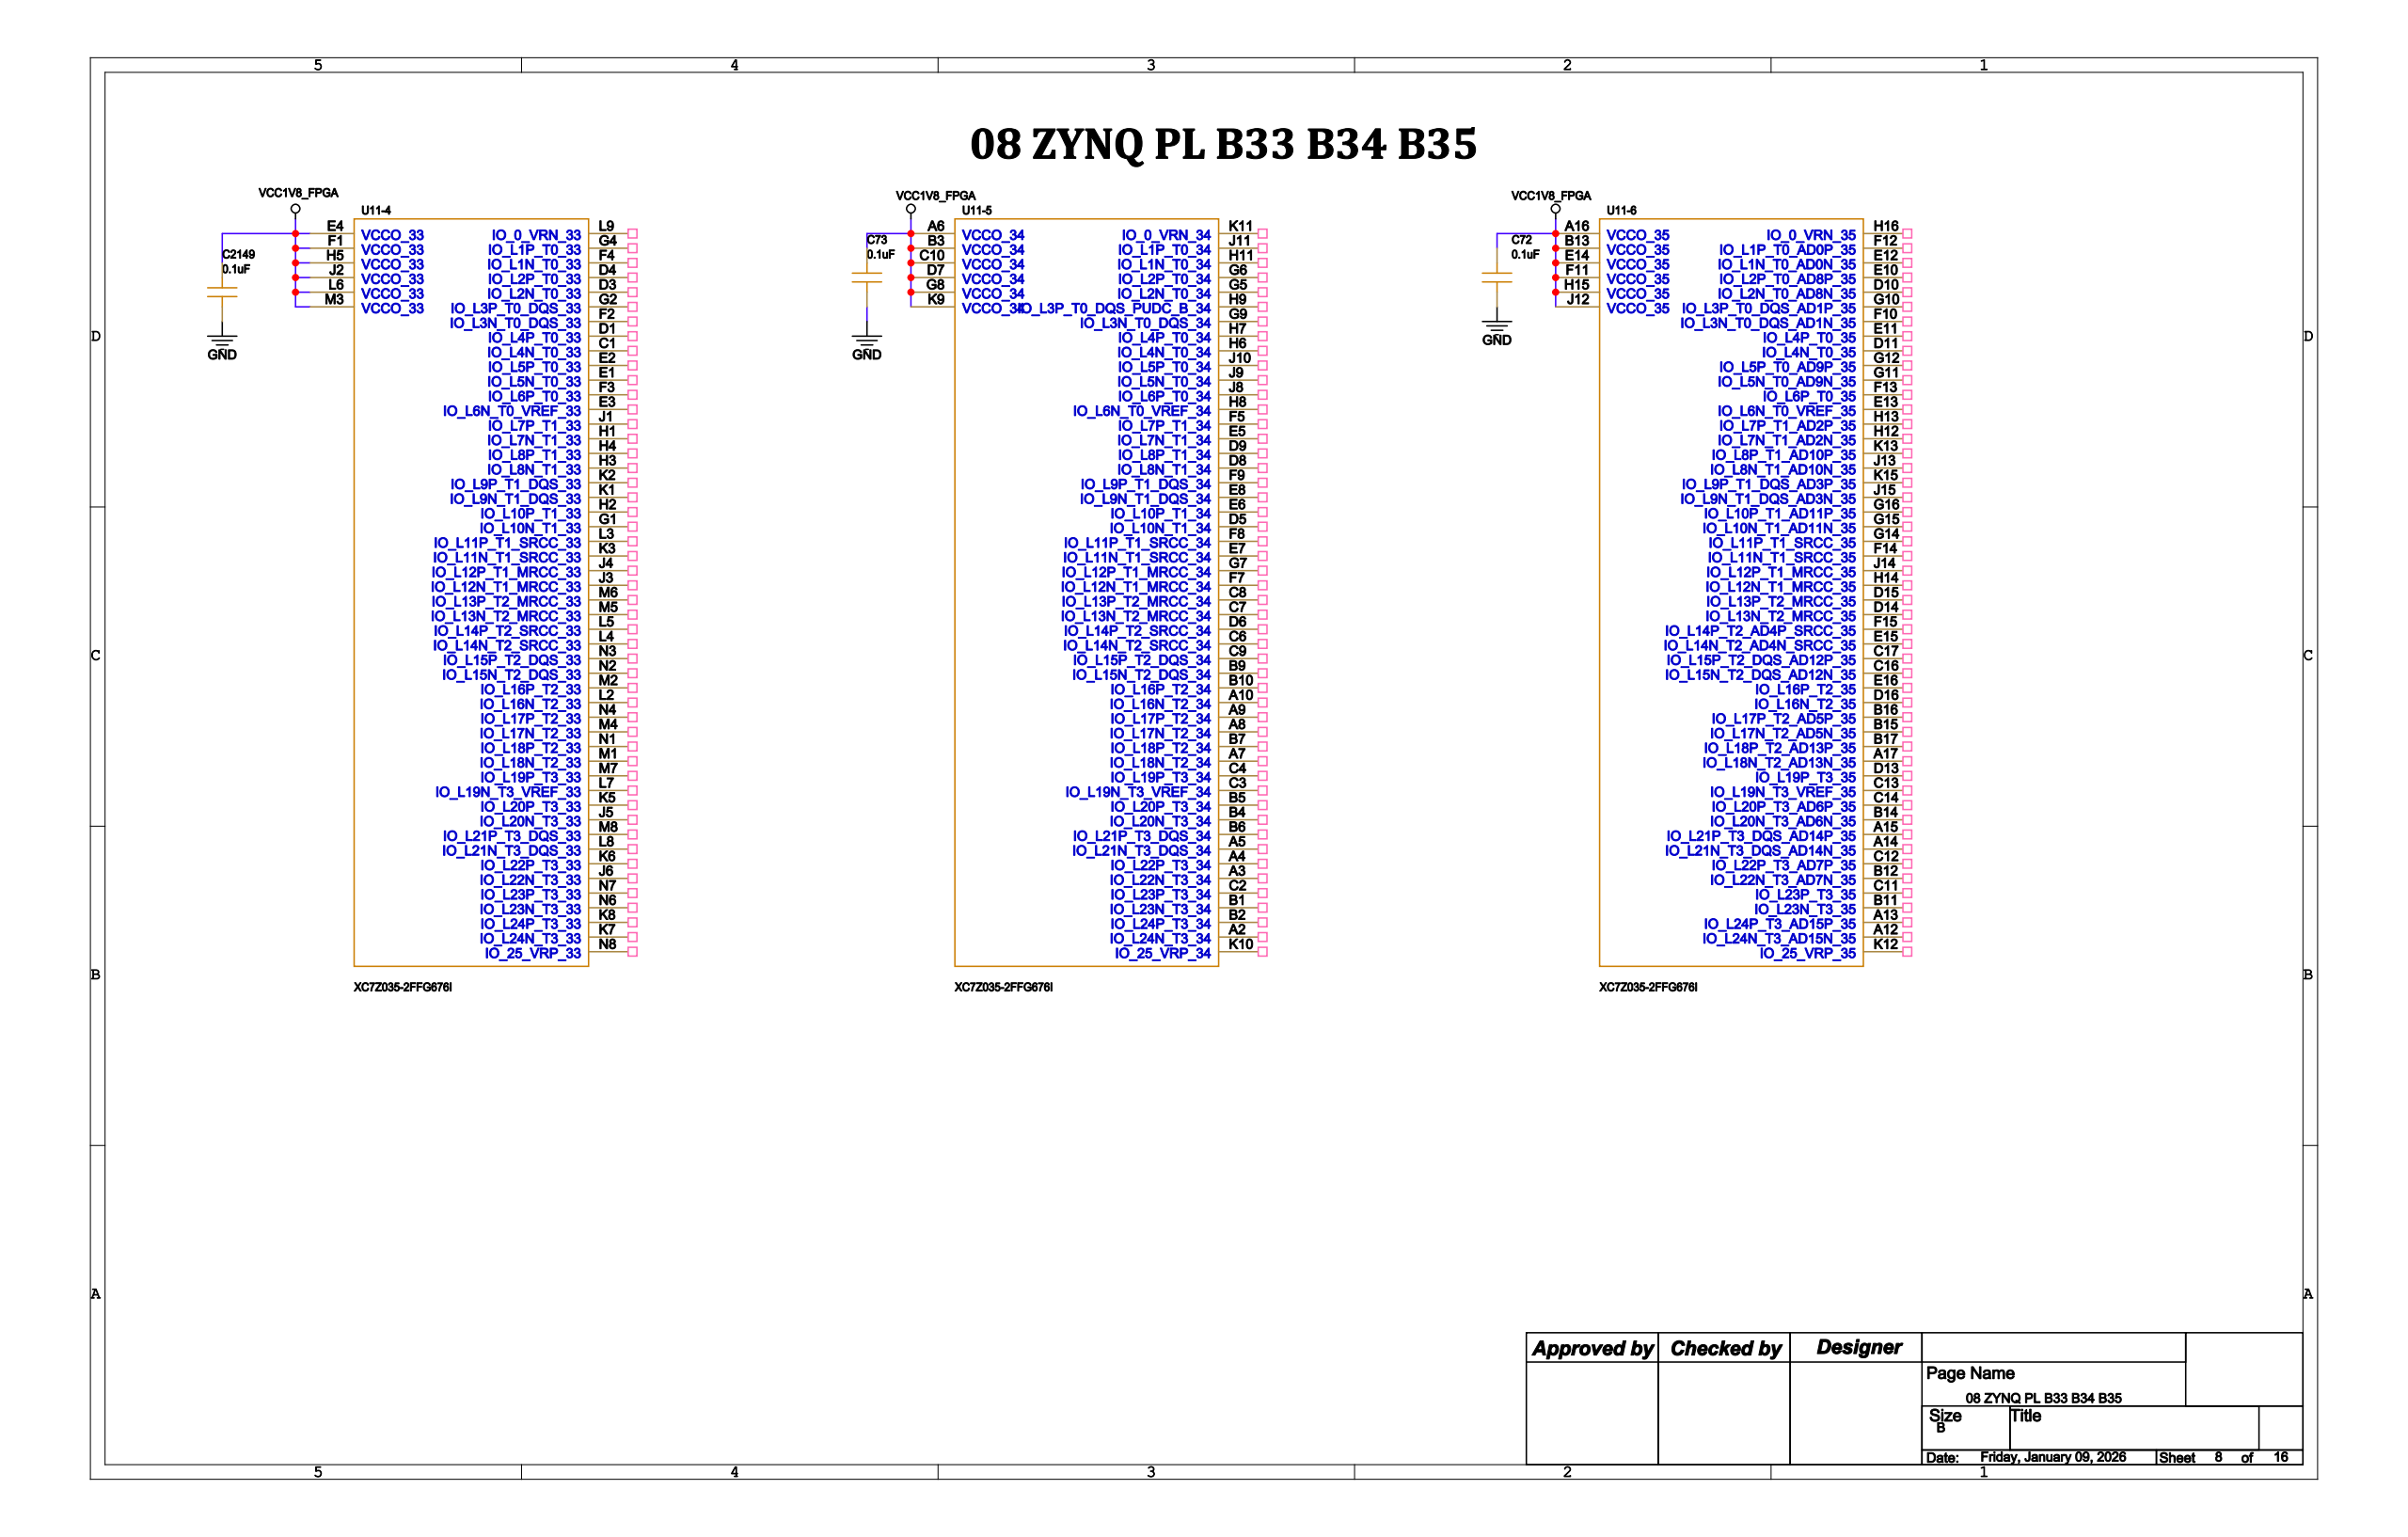Circuit board | Cadence Allegro | 442 parts | 326 nets | one sheet of the schematic
Parts on this sheet (reference | value | footprint):
C72 | 0.1uF | C0201
C73 | 0.1uF | C0201
C2149 | 0.1uF | C0201
Nets of these parts (net: part-pin ...):
GND: C72-2 C73-2 C2149-2
VCC1V8_FPGA: C72-1 C73-1 C2149-1